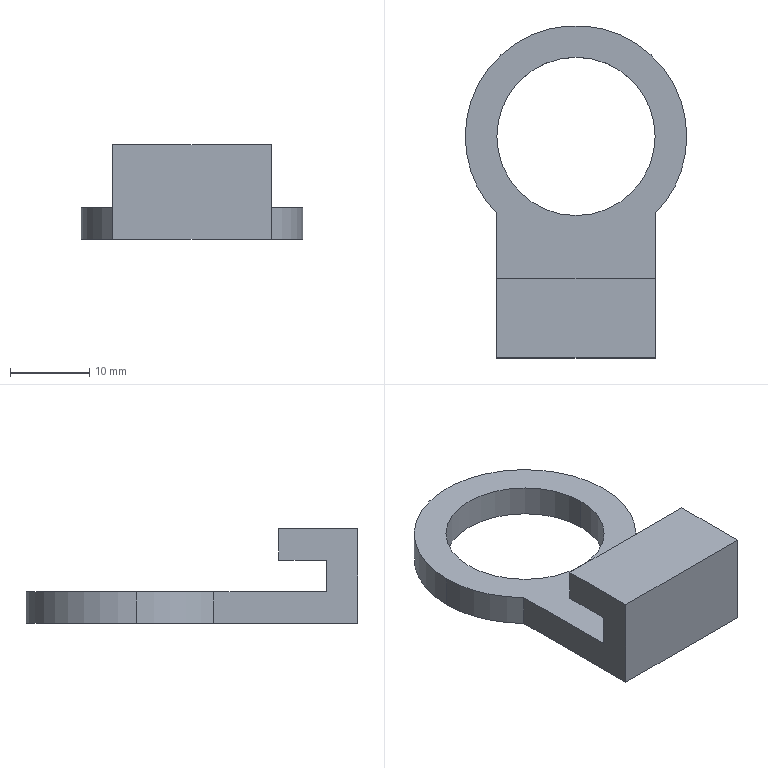Part | SolidWorks | features ICE 2, Extrusion 1, HoleWzd 1 | 1 solid | 14 faces | box 28 x 42 x 12 mm | volume 3551 mm3 | plane 9 | cylinder 5 | commonest cylinder face diameters 28 x3 20 x2
STEP:
#1=CARTESIAN_POINT('',(-10.,0.,0.));
#2=VERTEX_POINT('',#1);
#3=CARTESIAN_POINT('',(10.,0.,0.));
#4=VERTEX_POINT('',#3);
#5=CARTESIAN_POINT('',(0.,0.,0.));
#6=DIRECTION('',(0.,0.,1.));
#7=DIRECTION('',(1.,0.,0.));
#8=AXIS2_PLACEMENT_3D('',#5,#6,#7);
#9=CIRCLE('',#8,10.);
#10=EDGE_CURVE('',#2,#4,#9,.T.);
#11=ORIENTED_EDGE('',*,*,#10,.F.);
#12=CARTESIAN_POINT('',(-10.,0.,4.));
#13=VERTEX_POINT('',#12);
#14=CARTESIAN_POINT('',(-10.,0.,4.));
#15=DIRECTION('',(0.,0.,1.));
#16=VECTOR('',#15,1000.);
#17=LINE('',#14,#16);
#18=EDGE_CURVE('',#2,#13,#17,.T.);
#19=ORIENTED_EDGE('',*,*,#18,.T.);
#20=CARTESIAN_POINT('',(10.,0.,4.));
#21=VERTEX_POINT('',#20);
#22=CARTESIAN_POINT('',(0.,0.,4.));
#23=DIRECTION('',(0.,0.,1.));
#24=DIRECTION('',(1.,0.,0.));
#25=AXIS2_PLACEMENT_3D('',#22,#23,#24);
#26=CIRCLE('',#25,10.);
#27=EDGE_CURVE('',#13,#21,#26,.T.);
#28=ORIENTED_EDGE('',*,*,#27,.T.);
#29=CARTESIAN_POINT('',(10.,0.,4.));
#30=DIRECTION('',(0.,0.,1.));
#31=VECTOR('',#30,1000.);
#32=LINE('',#29,#31);
#33=EDGE_CURVE('',#4,#21,#32,.T.);
#34=ORIENTED_EDGE('',*,*,#33,.F.);
#35=EDGE_LOOP('',(#11,#19,#28,#34));
#36=FACE_OUTER_BOUND('',#35,.T.);
#37=CARTESIAN_POINT('',(0.,0.,4.));
#38=DIRECTION('',(0.,0.,1.));
#39=DIRECTION('',(1.,0.,0.));
#40=AXIS2_PLACEMENT_3D('',#37,#38,#39);
#41=CYLINDRICAL_SURFACE('',#40,10.);
#42=ADVANCED_FACE('',(#36),#41,.F.);
#43=CARTESIAN_POINT('',(-14.,0.,4.));
#44=VERTEX_POINT('',#43);
#45=CARTESIAN_POINT('',(14.,0.,4.));
#46=VERTEX_POINT('',#45);
#47=CARTESIAN_POINT('',(0.,0.,4.));
#48=DIRECTION('',(0.,0.,-1.));
#49=DIRECTION('',(-1.,0.,0.));
#50=AXIS2_PLACEMENT_3D('',#47,#48,#49);
#51=CIRCLE('',#50,14.);
#52=EDGE_CURVE('',#44,#46,#51,.T.);
#53=ORIENTED_EDGE('',*,*,#52,.T.);
#54=CARTESIAN_POINT('',(14.,0.,0.));
#55=VERTEX_POINT('',#54);
#56=CARTESIAN_POINT('',(14.,0.,4.));
#57=DIRECTION('',(0.,0.,-1.));
#58=VECTOR('',#57,1000.);
#59=LINE('',#56,#58);
#60=EDGE_CURVE('',#46,#55,#59,.T.);
#61=ORIENTED_EDGE('',*,*,#60,.T.);
#62=CARTESIAN_POINT('',(-14.,0.,0.));
#63=VERTEX_POINT('',#62);
#64=CARTESIAN_POINT('',(0.,0.,0.));
#65=DIRECTION('',(0.,0.,-1.));
#66=DIRECTION('',(-1.,0.,0.));
#67=AXIS2_PLACEMENT_3D('',#64,#65,#66);
#68=CIRCLE('',#67,14.);
#69=EDGE_CURVE('',#63,#55,#68,.T.);
#70=ORIENTED_EDGE('',*,*,#69,.F.);
#71=CARTESIAN_POINT('',(-14.,0.,4.));
#72=DIRECTION('',(0.,0.,-1.));
#73=VECTOR('',#72,1000.);
#74=LINE('',#71,#73);
#75=EDGE_CURVE('',#44,#63,#74,.T.);
#76=ORIENTED_EDGE('',*,*,#75,.F.);
#77=EDGE_LOOP('',(#53,#61,#70,#76));
#78=FACE_OUTER_BOUND('',#77,.T.);
#79=CARTESIAN_POINT('',(0.,0.,4.));
#80=DIRECTION('',(0.,0.,-1.));
#81=DIRECTION('',(-1.,0.,0.));
#82=AXIS2_PLACEMENT_3D('',#79,#80,#81);
#83=CYLINDRICAL_SURFACE('',#82,14.);
#84=ADVANCED_FACE('',(#78),#83,.T.);
#85=CARTESIAN_POINT('',(-10.,-9.798,4.));
#86=VERTEX_POINT('',#85);
#87=CARTESIAN_POINT('',(0.,0.,4.));
#88=DIRECTION('',(0.,0.,-1.));
#89=DIRECTION('',(-1.,0.,0.));
#90=AXIS2_PLACEMENT_3D('',#87,#88,#89);
#91=CIRCLE('',#90,14.);
#92=EDGE_CURVE('',#86,#44,#91,.T.);
#93=ORIENTED_EDGE('',*,*,#92,.T.);
#94=ORIENTED_EDGE('',*,*,#75,.T.);
#95=CARTESIAN_POINT('',(-10.,-9.798,0.));
#96=VERTEX_POINT('',#95);
#97=CARTESIAN_POINT('',(0.,0.,0.));
#98=DIRECTION('',(0.,0.,-1.));
#99=DIRECTION('',(-1.,0.,0.));
#100=AXIS2_PLACEMENT_3D('',#97,#98,#99);
#101=CIRCLE('',#100,14.);
#102=EDGE_CURVE('',#96,#63,#101,.T.);
#103=ORIENTED_EDGE('',*,*,#102,.F.);
#104=CARTESIAN_POINT('',(-10.,-9.798,4.));
#105=DIRECTION('',(0.,0.,-1.));
#106=VECTOR('',#105,1000.);
#107=LINE('',#104,#106);
#108=EDGE_CURVE('',#86,#96,#107,.T.);
#109=ORIENTED_EDGE('',*,*,#108,.F.);
#110=EDGE_LOOP('',(#93,#94,#103,#109));
#111=FACE_OUTER_BOUND('',#110,.T.);
#112=CARTESIAN_POINT('',(0.,0.,4.));
#113=DIRECTION('',(0.,0.,-1.));
#114=DIRECTION('',(-1.,0.,0.));
#115=AXIS2_PLACEMENT_3D('',#112,#113,#114);
#116=CYLINDRICAL_SURFACE('',#115,14.);
#117=ADVANCED_FACE('',(#111),#116,.T.);
#118=CARTESIAN_POINT('',(10.,-24.,8.));
#119=VERTEX_POINT('',#118);
#120=CARTESIAN_POINT('',(-10.,-24.,8.));
#121=VERTEX_POINT('',#120);
#122=CARTESIAN_POINT('',(-10.,-24.,8.));
#123=DIRECTION('',(-1.,0.,0.));
#124=VECTOR('',#123,1000.);
#125=LINE('',#122,#124);
#126=EDGE_CURVE('',#119,#121,#125,.T.);
#127=ORIENTED_EDGE('',*,*,#126,.F.);
#128=CARTESIAN_POINT('',(10.,-24.,4.));
#129=VERTEX_POINT('',#128);
#130=CARTESIAN_POINT('',(10.,-24.,12.));
#131=DIRECTION('',(0.,0.,-1.));
#132=VECTOR('',#131,1000.);
#133=LINE('',#130,#132);
#134=EDGE_CURVE('',#119,#129,#133,.T.);
#135=ORIENTED_EDGE('',*,*,#134,.T.);
#136=CARTESIAN_POINT('',(-10.,-24.,4.));
#137=VERTEX_POINT('',#136);
#138=CARTESIAN_POINT('',(-10.,-24.,4.));
#139=DIRECTION('',(-1.,0.,0.));
#140=VECTOR('',#139,1000.);
#141=LINE('',#138,#140);
#142=EDGE_CURVE('',#129,#137,#141,.T.);
#143=ORIENTED_EDGE('',*,*,#142,.T.);
#144=CARTESIAN_POINT('',(-10.,-24.,12.));
#145=DIRECTION('',(0.,0.,-1.));
#146=VECTOR('',#145,1000.);
#147=LINE('',#144,#146);
#148=EDGE_CURVE('',#121,#137,#147,.T.);
#149=ORIENTED_EDGE('',*,*,#148,.F.);
#150=EDGE_LOOP('',(#127,#135,#143,#149));
#151=FACE_OUTER_BOUND('',#150,.T.);
#152=CARTESIAN_POINT('',(-10.,-24.,12.));
#153=DIRECTION('',(0.,-1.,0.));
#154=DIRECTION('',(0.,0.,-1.));
#155=AXIS2_PLACEMENT_3D('',#152,#153,#154);
#156=PLANE('',#155);
#157=ADVANCED_FACE('',(#151),#156,.F.);
#158=CARTESIAN_POINT('',(0.,0.,4.));
#159=DIRECTION('',(0.,0.,1.));
#160=DIRECTION('',(1.,0.,0.));
#161=AXIS2_PLACEMENT_3D('',#158,#159,#160);
#162=CIRCLE('',#161,10.);
#163=EDGE_CURVE('',#21,#13,#162,.T.);
#164=ORIENTED_EDGE('',*,*,#163,.F.);
#165=ORIENTED_EDGE('',*,*,#27,.F.);
#166=EDGE_LOOP('',(#164,#165));
#167=FACE_BOUND('',#166,.T.);
#168=ORIENTED_EDGE('',*,*,#142,.F.);
#169=CARTESIAN_POINT('',(10.,-9.798,4.));
#170=VERTEX_POINT('',#169);
#171=CARTESIAN_POINT('',(10.,-9.798,4.));
#172=DIRECTION('',(0.,-1.,0.));
#173=VECTOR('',#172,1000.);
#174=LINE('',#171,#173);
#175=EDGE_CURVE('',#170,#129,#174,.T.);
#176=ORIENTED_EDGE('',*,*,#175,.F.);
#177=CARTESIAN_POINT('',(0.,0.,4.));
#178=DIRECTION('',(0.,0.,-1.));
#179=DIRECTION('',(-1.,0.,0.));
#180=AXIS2_PLACEMENT_3D('',#177,#178,#179);
#181=CIRCLE('',#180,14.);
#182=EDGE_CURVE('',#46,#170,#181,.T.);
#183=ORIENTED_EDGE('',*,*,#182,.F.);
#184=ORIENTED_EDGE('',*,*,#52,.F.);
#185=ORIENTED_EDGE('',*,*,#92,.F.);
#186=CARTESIAN_POINT('',(-10.,-28.,4.));
#187=DIRECTION('',(0.,1.,0.));
#188=VECTOR('',#187,1000.);
#189=LINE('',#186,#188);
#190=EDGE_CURVE('',#137,#86,#189,.T.);
#191=ORIENTED_EDGE('',*,*,#190,.F.);
#192=EDGE_LOOP('',(#168,#176,#183,#184,#185,#191));
#193=FACE_OUTER_BOUND('',#192,.T.);
#194=CARTESIAN_POINT('',(0.,0.,4.));
#195=DIRECTION('',(0.,0.,-1.));
#196=DIRECTION('',(-1.,0.,0.));
#197=AXIS2_PLACEMENT_3D('',#194,#195,#196);
#198=PLANE('',#197);
#199=ADVANCED_FACE('',(#167,#193),#198,.F.);
#200=CARTESIAN_POINT('',(10.,-9.798,0.));
#201=VERTEX_POINT('',#200);
#202=CARTESIAN_POINT('',(10.,-28.,0.));
#203=VERTEX_POINT('',#202);
#204=CARTESIAN_POINT('',(10.,-9.798,0.));
#205=DIRECTION('',(0.,-1.,0.));
#206=VECTOR('',#205,1000.);
#207=LINE('',#204,#206);
#208=EDGE_CURVE('',#201,#203,#207,.T.);
#209=ORIENTED_EDGE('',*,*,#208,.F.);
#210=CARTESIAN_POINT('',(10.,-9.798,4.));
#211=DIRECTION('',(0.,0.,-1.));
#212=VECTOR('',#211,1000.);
#213=LINE('',#210,#212);
#214=EDGE_CURVE('',#170,#201,#213,.T.);
#215=ORIENTED_EDGE('',*,*,#214,.F.);
#216=ORIENTED_EDGE('',*,*,#175,.T.);
#217=ORIENTED_EDGE('',*,*,#134,.F.);
#218=CARTESIAN_POINT('',(10.,-18.,8.));
#219=VERTEX_POINT('',#218);
#220=CARTESIAN_POINT('',(10.,-18.,8.));
#221=DIRECTION('',(0.,-1.,0.));
#222=VECTOR('',#221,1000.);
#223=LINE('',#220,#222);
#224=EDGE_CURVE('',#219,#119,#223,.T.);
#225=ORIENTED_EDGE('',*,*,#224,.F.);
#226=CARTESIAN_POINT('',(10.,-18.,12.));
#227=VERTEX_POINT('',#226);
#228=CARTESIAN_POINT('',(10.,-18.,8.));
#229=DIRECTION('',(0.,0.,-1.));
#230=VECTOR('',#229,1000.);
#231=LINE('',#228,#230);
#232=EDGE_CURVE('',#227,#219,#231,.T.);
#233=ORIENTED_EDGE('',*,*,#232,.F.);
#234=CARTESIAN_POINT('',(10.,-28.,12.));
#235=VERTEX_POINT('',#234);
#236=CARTESIAN_POINT('',(10.,-24.,12.));
#237=DIRECTION('',(0.,1.,0.));
#238=VECTOR('',#237,1000.);
#239=LINE('',#236,#238);
#240=EDGE_CURVE('',#235,#227,#239,.T.);
#241=ORIENTED_EDGE('',*,*,#240,.F.);
#242=CARTESIAN_POINT('',(10.,-28.,4.));
#243=DIRECTION('',(0.,0.,-1.));
#244=VECTOR('',#243,1000.);
#245=LINE('',#242,#244);
#246=EDGE_CURVE('',#235,#203,#245,.T.);
#247=ORIENTED_EDGE('',*,*,#246,.T.);
#248=EDGE_LOOP('',(#209,#215,#216,#217,#225,#233,#241,#247));
#249=FACE_OUTER_BOUND('',#248,.T.);
#250=CARTESIAN_POINT('',(10.,-9.798,4.));
#251=DIRECTION('',(1.,0.,0.));
#252=DIRECTION('',(0.,0.,-1.));
#253=AXIS2_PLACEMENT_3D('',#250,#251,#252);
#254=PLANE('',#253);
#255=ADVANCED_FACE('',(#249),#254,.T.);
#256=ORIENTED_EDGE('',*,*,#60,.F.);
#257=ORIENTED_EDGE('',*,*,#182,.T.);
#258=ORIENTED_EDGE('',*,*,#214,.T.);
#259=CARTESIAN_POINT('',(0.,0.,0.));
#260=DIRECTION('',(0.,0.,-1.));
#261=DIRECTION('',(-1.,0.,0.));
#262=AXIS2_PLACEMENT_3D('',#259,#260,#261);
#263=CIRCLE('',#262,14.);
#264=EDGE_CURVE('',#55,#201,#263,.T.);
#265=ORIENTED_EDGE('',*,*,#264,.F.);
#266=EDGE_LOOP('',(#256,#257,#258,#265));
#267=FACE_OUTER_BOUND('',#266,.T.);
#268=CARTESIAN_POINT('',(0.,0.,4.));
#269=DIRECTION('',(0.,0.,-1.));
#270=DIRECTION('',(-1.,0.,0.));
#271=AXIS2_PLACEMENT_3D('',#268,#269,#270);
#272=CYLINDRICAL_SURFACE('',#271,14.);
#273=ADVANCED_FACE('',(#267),#272,.T.);
#274=CARTESIAN_POINT('',(-10.,-28.,0.));
#275=VERTEX_POINT('',#274);
#276=CARTESIAN_POINT('',(-10.,-28.,0.));
#277=DIRECTION('',(0.,1.,0.));
#278=VECTOR('',#277,1000.);
#279=LINE('',#276,#278);
#280=EDGE_CURVE('',#275,#96,#279,.T.);
#281=ORIENTED_EDGE('',*,*,#280,.F.);
#282=CARTESIAN_POINT('',(-10.,-28.,12.));
#283=VERTEX_POINT('',#282);
#284=CARTESIAN_POINT('',(-10.,-28.,4.));
#285=DIRECTION('',(0.,0.,-1.));
#286=VECTOR('',#285,1000.);
#287=LINE('',#284,#286);
#288=EDGE_CURVE('',#283,#275,#287,.T.);
#289=ORIENTED_EDGE('',*,*,#288,.F.);
#290=CARTESIAN_POINT('',(-10.,-18.,12.));
#291=VERTEX_POINT('',#290);
#292=CARTESIAN_POINT('',(-10.,-28.,12.));
#293=DIRECTION('',(0.,-1.,0.));
#294=VECTOR('',#293,1000.);
#295=LINE('',#292,#294);
#296=EDGE_CURVE('',#291,#283,#295,.T.);
#297=ORIENTED_EDGE('',*,*,#296,.F.);
#298=CARTESIAN_POINT('',(-10.,-18.,8.));
#299=VERTEX_POINT('',#298);
#300=CARTESIAN_POINT('',(-10.,-18.,12.));
#301=DIRECTION('',(0.,0.,1.));
#302=VECTOR('',#301,1000.);
#303=LINE('',#300,#302);
#304=EDGE_CURVE('',#299,#291,#303,.T.);
#305=ORIENTED_EDGE('',*,*,#304,.F.);
#306=CARTESIAN_POINT('',(-10.,-18.,8.));
#307=DIRECTION('',(0.,-1.,0.));
#308=VECTOR('',#307,1000.);
#309=LINE('',#306,#308);
#310=EDGE_CURVE('',#299,#121,#309,.T.);
#311=ORIENTED_EDGE('',*,*,#310,.T.);
#312=ORIENTED_EDGE('',*,*,#148,.T.);
#313=ORIENTED_EDGE('',*,*,#190,.T.);
#314=ORIENTED_EDGE('',*,*,#108,.T.);
#315=EDGE_LOOP('',(#281,#289,#297,#305,#311,#312,#313,#314));
#316=FACE_OUTER_BOUND('',#315,.T.);
#317=CARTESIAN_POINT('',(-10.,-28.,4.));
#318=DIRECTION('',(-1.,0.,0.));
#319=DIRECTION('',(0.,0.,1.));
#320=AXIS2_PLACEMENT_3D('',#317,#318,#319);
#321=PLANE('',#320);
#322=ADVANCED_FACE('',(#316),#321,.T.);
#323=CARTESIAN_POINT('',(10.,-28.,0.));
#324=DIRECTION('',(-1.,0.,0.));
#325=VECTOR('',#324,1000.);
#326=LINE('',#323,#325);
#327=EDGE_CURVE('',#203,#275,#326,.T.);
#328=ORIENTED_EDGE('',*,*,#327,.F.);
#329=ORIENTED_EDGE('',*,*,#246,.F.);
#330=CARTESIAN_POINT('',(10.,-28.,12.));
#331=DIRECTION('',(1.,0.,0.));
#332=VECTOR('',#331,1000.);
#333=LINE('',#330,#332);
#334=EDGE_CURVE('',#283,#235,#333,.T.);
#335=ORIENTED_EDGE('',*,*,#334,.F.);
#336=ORIENTED_EDGE('',*,*,#288,.T.);
#337=EDGE_LOOP('',(#328,#329,#335,#336));
#338=FACE_OUTER_BOUND('',#337,.T.);
#339=CARTESIAN_POINT('',(10.,-28.,4.));
#340=DIRECTION('',(0.,-1.,0.));
#341=DIRECTION('',(0.,0.,-1.));
#342=AXIS2_PLACEMENT_3D('',#339,#340,#341);
#343=PLANE('',#342);
#344=ADVANCED_FACE('',(#338),#343,.T.);
#345=CARTESIAN_POINT('',(0.,0.,0.));
#346=DIRECTION('',(0.,0.,1.));
#347=DIRECTION('',(1.,0.,0.));
#348=AXIS2_PLACEMENT_3D('',#345,#346,#347);
#349=CIRCLE('',#348,10.);
#350=EDGE_CURVE('',#4,#2,#349,.T.);
#351=ORIENTED_EDGE('',*,*,#350,.T.);
#352=ORIENTED_EDGE('',*,*,#10,.T.);
#353=EDGE_LOOP('',(#351,#352));
#354=FACE_BOUND('',#353,.T.);
#355=ORIENTED_EDGE('',*,*,#208,.T.);
#356=ORIENTED_EDGE('',*,*,#327,.T.);
#357=ORIENTED_EDGE('',*,*,#280,.T.);
#358=ORIENTED_EDGE('',*,*,#102,.T.);
#359=ORIENTED_EDGE('',*,*,#69,.T.);
#360=ORIENTED_EDGE('',*,*,#264,.T.);
#361=EDGE_LOOP('',(#355,#356,#357,#358,#359,#360));
#362=FACE_OUTER_BOUND('',#361,.T.);
#363=CARTESIAN_POINT('',(0.,0.,0.));
#364=DIRECTION('',(0.,0.,-1.));
#365=DIRECTION('',(-1.,0.,0.));
#366=AXIS2_PLACEMENT_3D('',#363,#364,#365);
#367=PLANE('',#366);
#368=ADVANCED_FACE('',(#354,#362),#367,.T.);
#369=ORIENTED_EDGE('',*,*,#240,.T.);
#370=CARTESIAN_POINT('',(10.,-18.,12.));
#371=DIRECTION('',(1.,0.,0.));
#372=VECTOR('',#371,1000.);
#373=LINE('',#370,#372);
#374=EDGE_CURVE('',#291,#227,#373,.T.);
#375=ORIENTED_EDGE('',*,*,#374,.F.);
#376=ORIENTED_EDGE('',*,*,#296,.T.);
#377=ORIENTED_EDGE('',*,*,#334,.T.);
#378=EDGE_LOOP('',(#369,#375,#376,#377));
#379=FACE_OUTER_BOUND('',#378,.T.);
#380=CARTESIAN_POINT('',(0.,0.,12.));
#381=DIRECTION('',(0.,0.,-1.));
#382=DIRECTION('',(-1.,0.,0.));
#383=AXIS2_PLACEMENT_3D('',#380,#381,#382);
#384=PLANE('',#383);
#385=ADVANCED_FACE('',(#379),#384,.F.);
#386=ORIENTED_EDGE('',*,*,#126,.T.);
#387=ORIENTED_EDGE('',*,*,#310,.F.);
#388=CARTESIAN_POINT('',(-10.,-18.,8.));
#389=DIRECTION('',(-1.,0.,0.));
#390=VECTOR('',#389,1000.);
#391=LINE('',#388,#390);
#392=EDGE_CURVE('',#219,#299,#391,.T.);
#393=ORIENTED_EDGE('',*,*,#392,.F.);
#394=ORIENTED_EDGE('',*,*,#224,.T.);
#395=EDGE_LOOP('',(#386,#387,#393,#394));
#396=FACE_OUTER_BOUND('',#395,.T.);
#397=CARTESIAN_POINT('',(-10.,-18.,8.));
#398=DIRECTION('',(0.,0.,1.));
#399=DIRECTION('',(1.,0.,0.));
#400=AXIS2_PLACEMENT_3D('',#397,#398,#399);
#401=PLANE('',#400);
#402=ADVANCED_FACE('',(#396),#401,.F.);
#403=ORIENTED_EDGE('',*,*,#392,.T.);
#404=ORIENTED_EDGE('',*,*,#304,.T.);
#405=ORIENTED_EDGE('',*,*,#374,.T.);
#406=ORIENTED_EDGE('',*,*,#232,.T.);
#407=EDGE_LOOP('',(#403,#404,#405,#406));
#408=FACE_OUTER_BOUND('',#407,.T.);
#409=CARTESIAN_POINT('',(0.,-18.,0.));
#410=DIRECTION('',(0.,-1.,0.));
#411=DIRECTION('',(0.,0.,-1.));
#412=AXIS2_PLACEMENT_3D('',#409,#410,#411);
#413=PLANE('',#412);
#414=ADVANCED_FACE('',(#408),#413,.F.);
#415=ORIENTED_EDGE('',*,*,#18,.F.);
#416=ORIENTED_EDGE('',*,*,#350,.F.);
#417=ORIENTED_EDGE('',*,*,#33,.T.);
#418=ORIENTED_EDGE('',*,*,#163,.T.);
#419=EDGE_LOOP('',(#415,#416,#417,#418));
#420=FACE_OUTER_BOUND('',#419,.T.);
#421=CARTESIAN_POINT('',(0.,0.,4.));
#422=DIRECTION('',(0.,0.,1.));
#423=DIRECTION('',(1.,0.,0.));
#424=AXIS2_PLACEMENT_3D('',#421,#422,#423);
#425=CYLINDRICAL_SURFACE('',#424,10.);
#426=ADVANCED_FACE('',(#420),#425,.F.);
#427=CLOSED_SHELL('',(#42,#84,#117,#157,#199,#255,#273,#322,#344,#368,#385,#402,#414,#426));
#428=MANIFOLD_SOLID_BREP('',#427);
#429=CARTESIAN_POINT('',(0.,0.,0.));
#430=DIRECTION('',(0.,0.,1.));
#431=DIRECTION('',(1.,0.,0.));
#432=AXIS2_PLACEMENT_3D('',#429,#430,#431);
#433=(LENGTH_UNIT()NAMED_UNIT(*)SI_UNIT(.MILLI.,.METRE.));
#434=UNCERTAINTY_MEASURE_WITH_UNIT(LENGTH_MEASURE(0.00001),#433,'','');
#435=(NAMED_UNIT(*)PLANE_ANGLE_UNIT()SI_UNIT($,.RADIAN.));
#436=(NAMED_UNIT(*)SI_UNIT($,.STERADIAN.)SOLID_ANGLE_UNIT());
#437=(GEOMETRIC_REPRESENTATION_CONTEXT(3)GLOBAL_UNCERTAINTY_ASSIGNED_CONTEXT((#434))GLOBAL_UNIT_ASSIGNED_CONTEXT((#433,#435,#436))REPRESENTATION_CONTEXT('',''));
#438=ADVANCED_BREP_SHAPE_REPRESENTATION('',(#428,#432),#437);